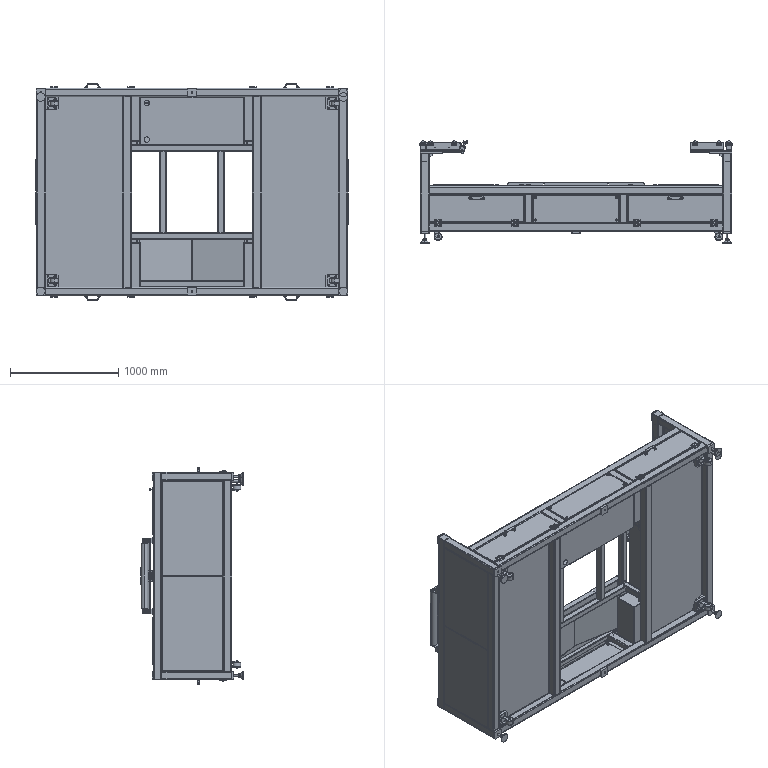Part | SolidWorks | 238 solids | 6442 faces | volume 79648659 mm3 | plane 3041 | cylinder 2835 | cone 242 | torus 186 | spline 132 | sphere 6 | commonest cylinder face diameters 6.8 x464 10 x250 7 x248 5 x219 3.3 x178 20 x152